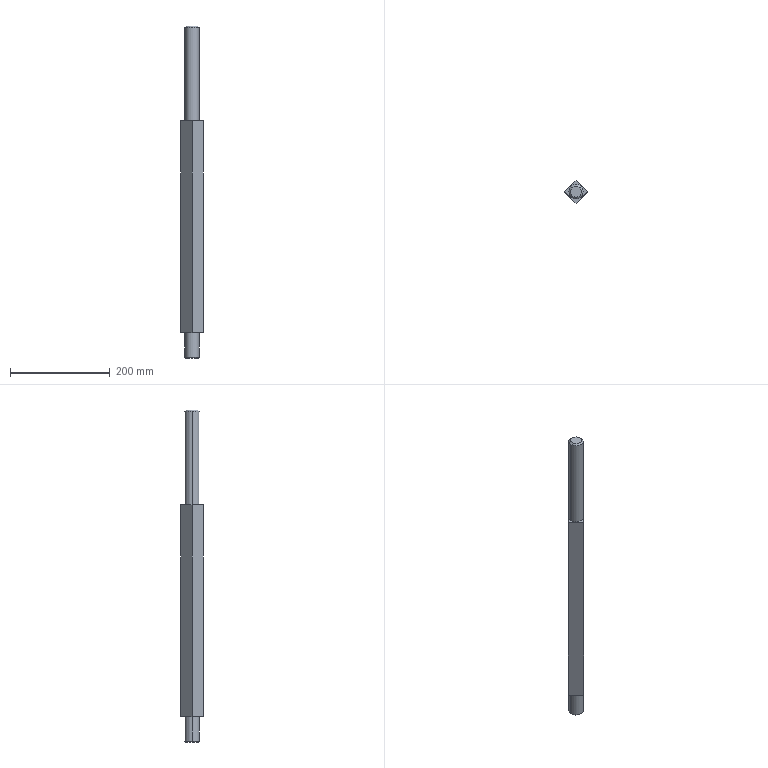Part | SolidWorks | features Chamfer 2, Extrusion 1, RevCut 1 | 1 solid | 16 faces | box 45.255 x 45.255 x 664.7 mm | volume 588102 mm3 | plane 8 | cone 4 | cylinder 4 | commonest cylinder face diameters 28.575 x4
STEP:
#1=CARTESIAN_POINT('',(11.287,0.,664.7));
#2=VERTEX_POINT('',#1);
#3=CARTESIAN_POINT('',(-11.287,0.,664.7));
#4=VERTEX_POINT('',#3);
#5=CARTESIAN_POINT('',(0.,0.,664.7));
#6=DIRECTION('',(0.,0.,1.));
#7=DIRECTION('',(1.,0.,0.));
#8=AXIS2_PLACEMENT_3D('',#5,#6,#7);
#9=CIRCLE('',#8,11.287);
#10=EDGE_CURVE('',#2,#4,#9,.T.);
#11=ORIENTED_EDGE('',*,*,#10,.F.);
#12=CARTESIAN_POINT('',(14.288,0.,661.7));
#13=VERTEX_POINT('',#12);
#14=CARTESIAN_POINT('',(14.288,0.,661.7));
#15=DIRECTION('',(0.7071,0.,-0.7071));
#16=VECTOR('',#15,1000.);
#17=LINE('',#14,#16);
#18=EDGE_CURVE('',#2,#13,#17,.T.);
#19=ORIENTED_EDGE('',*,*,#18,.T.);
#20=CARTESIAN_POINT('',(-14.288,0.,661.7));
#21=VERTEX_POINT('',#20);
#22=CARTESIAN_POINT('',(0.,0.,661.7));
#23=DIRECTION('',(0.,0.,-1.));
#24=DIRECTION('',(1.,0.,0.));
#25=AXIS2_PLACEMENT_3D('',#22,#23,#24);
#26=CIRCLE('',#25,14.288);
#27=EDGE_CURVE('',#21,#13,#26,.T.);
#28=ORIENTED_EDGE('',*,*,#27,.F.);
#29=CARTESIAN_POINT('',(-14.288,0.,661.7));
#30=DIRECTION('',(-0.7071,0.,-0.7071));
#31=VECTOR('',#30,1000.);
#32=LINE('',#29,#31);
#33=EDGE_CURVE('',#4,#21,#32,.T.);
#34=ORIENTED_EDGE('',*,*,#33,.F.);
#35=EDGE_LOOP('',(#11,#19,#28,#34));
#36=FACE_OUTER_BOUND('',#35,.T.);
#37=CARTESIAN_POINT('',(0.,0.,661.7));
#38=DIRECTION('',(0.,0.,-1.));
#39=DIRECTION('',(-1.,0.,0.));
#40=AXIS2_PLACEMENT_3D('',#37,#38,#39);
#41=CONICAL_SURFACE('',#40,14.288,0.7854);
#42=ADVANCED_FACE('',(#36),#41,.T.);
#43=CARTESIAN_POINT('',(-12.787,0.,0.));
#44=VERTEX_POINT('',#43);
#45=CARTESIAN_POINT('',(12.787,0.,0.));
#46=VERTEX_POINT('',#45);
#47=CARTESIAN_POINT('',(0.,0.,0.));
#48=DIRECTION('',(0.,0.,-1.));
#49=DIRECTION('',(1.,0.,0.));
#50=AXIS2_PLACEMENT_3D('',#47,#48,#49);
#51=CIRCLE('',#50,12.787);
#52=EDGE_CURVE('',#44,#46,#51,.T.);
#53=ORIENTED_EDGE('',*,*,#52,.F.);
#54=CARTESIAN_POINT('',(-14.288,0.,1.5));
#55=VERTEX_POINT('',#54);
#56=CARTESIAN_POINT('',(-12.787,0.,0.));
#57=DIRECTION('',(-0.7071,0.,0.7071));
#58=VECTOR('',#57,1000.);
#59=LINE('',#56,#58);
#60=EDGE_CURVE('',#44,#55,#59,.T.);
#61=ORIENTED_EDGE('',*,*,#60,.T.);
#62=CARTESIAN_POINT('',(14.288,0.,1.5));
#63=VERTEX_POINT('',#62);
#64=CARTESIAN_POINT('',(0.,0.,1.5));
#65=DIRECTION('',(0.,0.,1.));
#66=DIRECTION('',(1.,0.,0.));
#67=AXIS2_PLACEMENT_3D('',#64,#65,#66);
#68=CIRCLE('',#67,14.288);
#69=EDGE_CURVE('',#63,#55,#68,.T.);
#70=ORIENTED_EDGE('',*,*,#69,.F.);
#71=CARTESIAN_POINT('',(12.787,0.,0.));
#72=DIRECTION('',(0.7071,0.,0.7071));
#73=VECTOR('',#72,1000.);
#74=LINE('',#71,#73);
#75=EDGE_CURVE('',#46,#63,#74,.T.);
#76=ORIENTED_EDGE('',*,*,#75,.F.);
#77=EDGE_LOOP('',(#53,#61,#70,#76));
#78=FACE_OUTER_BOUND('',#77,.T.);
#79=CARTESIAN_POINT('',(0.,0.,0.));
#80=DIRECTION('',(0.,0.,1.));
#81=DIRECTION('',(1.,0.,0.));
#82=AXIS2_PLACEMENT_3D('',#79,#80,#81);
#83=CONICAL_SURFACE('',#82,12.787,0.7854);
#84=ADVANCED_FACE('',(#78),#83,.T.);
#85=ORIENTED_EDGE('',*,*,#27,.T.);
#86=CARTESIAN_POINT('',(14.288,0.,474.9));
#87=VERTEX_POINT('',#86);
#88=CARTESIAN_POINT('',(14.288,0.,0.));
#89=DIRECTION('',(0.,0.,-1.));
#90=VECTOR('',#89,1000.);
#91=LINE('',#88,#90);
#92=EDGE_CURVE('',#13,#87,#91,.T.);
#93=ORIENTED_EDGE('',*,*,#92,.T.);
#94=CARTESIAN_POINT('',(-14.288,0.,474.9));
#95=VERTEX_POINT('',#94);
#96=CARTESIAN_POINT('',(0.,0.,474.9));
#97=DIRECTION('',(0.,0.,-1.));
#98=DIRECTION('',(-1.,0.,0.));
#99=AXIS2_PLACEMENT_3D('',#96,#97,#98);
#100=CIRCLE('',#99,14.288);
#101=EDGE_CURVE('',#95,#87,#100,.T.);
#102=ORIENTED_EDGE('',*,*,#101,.F.);
#103=CARTESIAN_POINT('',(-14.288,0.,0.));
#104=DIRECTION('',(0.,0.,-1.));
#105=VECTOR('',#104,1000.);
#106=LINE('',#103,#105);
#107=EDGE_CURVE('',#21,#95,#106,.T.);
#108=ORIENTED_EDGE('',*,*,#107,.F.);
#109=EDGE_LOOP('',(#85,#93,#102,#108));
#110=FACE_OUTER_BOUND('',#109,.T.);
#111=CARTESIAN_POINT('',(0.,0.,0.));
#112=DIRECTION('',(0.,0.,-1.));
#113=DIRECTION('',(-1.,0.,0.));
#114=AXIS2_PLACEMENT_3D('',#111,#112,#113);
#115=CYLINDRICAL_SURFACE('',#114,14.288);
#116=ADVANCED_FACE('',(#110),#115,.T.);
#117=CARTESIAN_POINT('',(-14.288,0.,50.8));
#118=VERTEX_POINT('',#117);
#119=CARTESIAN_POINT('',(14.288,0.,50.8));
#120=VERTEX_POINT('',#119);
#121=CARTESIAN_POINT('',(0.,0.,50.8));
#122=DIRECTION('',(0.,0.,-1.));
#123=DIRECTION('',(-1.,0.,0.));
#124=AXIS2_PLACEMENT_3D('',#121,#122,#123);
#125=CIRCLE('',#124,14.288);
#126=EDGE_CURVE('',#118,#120,#125,.T.);
#127=ORIENTED_EDGE('',*,*,#126,.T.);
#128=CARTESIAN_POINT('',(14.288,0.,0.));
#129=DIRECTION('',(0.,0.,-1.));
#130=VECTOR('',#129,1000.);
#131=LINE('',#128,#130);
#132=EDGE_CURVE('',#120,#63,#131,.T.);
#133=ORIENTED_EDGE('',*,*,#132,.T.);
#134=ORIENTED_EDGE('',*,*,#69,.T.);
#135=CARTESIAN_POINT('',(-14.288,0.,0.));
#136=DIRECTION('',(0.,0.,-1.));
#137=VECTOR('',#136,1000.);
#138=LINE('',#135,#137);
#139=EDGE_CURVE('',#118,#55,#138,.T.);
#140=ORIENTED_EDGE('',*,*,#139,.F.);
#141=EDGE_LOOP('',(#127,#133,#134,#140));
#142=FACE_OUTER_BOUND('',#141,.T.);
#143=CARTESIAN_POINT('',(0.,0.,0.));
#144=DIRECTION('',(0.,0.,-1.));
#145=DIRECTION('',(-1.,0.,0.));
#146=AXIS2_PLACEMENT_3D('',#143,#144,#145);
#147=CYLINDRICAL_SURFACE('',#146,14.288);
#148=ADVANCED_FACE('',(#142),#147,.T.);
#149=CARTESIAN_POINT('',(-22.627,0.,474.9));
#150=VERTEX_POINT('',#149);
#151=CARTESIAN_POINT('',(0.,-22.627,474.9));
#152=VERTEX_POINT('',#151);
#153=CARTESIAN_POINT('',(-22.627,0.,474.9));
#154=DIRECTION('',(0.7071,-0.7071,0.));
#155=VECTOR('',#154,1000.);
#156=LINE('',#153,#155);
#157=EDGE_CURVE('',#150,#152,#156,.T.);
#158=ORIENTED_EDGE('',*,*,#157,.F.);
#159=CARTESIAN_POINT('',(-22.627,0.,50.8));
#160=VERTEX_POINT('',#159);
#161=CARTESIAN_POINT('',(-22.627,0.,664.7));
#162=DIRECTION('',(0.,0.,-1.));
#163=VECTOR('',#162,1000.);
#164=LINE('',#161,#163);
#165=EDGE_CURVE('',#150,#160,#164,.T.);
#166=ORIENTED_EDGE('',*,*,#165,.T.);
#167=CARTESIAN_POINT('',(0.,-22.627,50.8));
#168=VERTEX_POINT('',#167);
#169=CARTESIAN_POINT('',(-22.627,0.,50.8));
#170=DIRECTION('',(-0.7071,0.7071,0.));
#171=VECTOR('',#170,1000.);
#172=LINE('',#169,#171);
#173=EDGE_CURVE('',#168,#160,#172,.T.);
#174=ORIENTED_EDGE('',*,*,#173,.F.);
#175=CARTESIAN_POINT('',(0.,-22.627,664.7));
#176=DIRECTION('',(0.,0.,-1.));
#177=VECTOR('',#176,1000.);
#178=LINE('',#175,#177);
#179=EDGE_CURVE('',#152,#168,#178,.T.);
#180=ORIENTED_EDGE('',*,*,#179,.F.);
#181=EDGE_LOOP('',(#158,#166,#174,#180));
#182=FACE_OUTER_BOUND('',#181,.T.);
#183=CARTESIAN_POINT('',(-22.627,0.,664.7));
#184=DIRECTION('',(0.7071,0.7071,0.));
#185=DIRECTION('',(-0.7071,0.7071,0.));
#186=AXIS2_PLACEMENT_3D('',#183,#184,#185);
#187=PLANE('',#186);
#188=ADVANCED_FACE('',(#182),#187,.F.);
#189=CARTESIAN_POINT('',(22.627,0.,474.9));
#190=VERTEX_POINT('',#189);
#191=CARTESIAN_POINT('',(0.,-22.627,474.9));
#192=DIRECTION('',(0.7071,0.7071,0.));
#193=VECTOR('',#192,1000.);
#194=LINE('',#191,#193);
#195=EDGE_CURVE('',#152,#190,#194,.T.);
#196=ORIENTED_EDGE('',*,*,#195,.F.);
#197=ORIENTED_EDGE('',*,*,#179,.T.);
#198=CARTESIAN_POINT('',(22.627,0.,50.8));
#199=VERTEX_POINT('',#198);
#200=CARTESIAN_POINT('',(0.,-22.627,50.8));
#201=DIRECTION('',(-0.7071,-0.7071,0.));
#202=VECTOR('',#201,1000.);
#203=LINE('',#200,#202);
#204=EDGE_CURVE('',#199,#168,#203,.T.);
#205=ORIENTED_EDGE('',*,*,#204,.F.);
#206=CARTESIAN_POINT('',(22.627,0.,664.7));
#207=DIRECTION('',(0.,0.,-1.));
#208=VECTOR('',#207,1000.);
#209=LINE('',#206,#208);
#210=EDGE_CURVE('',#190,#199,#209,.T.);
#211=ORIENTED_EDGE('',*,*,#210,.F.);
#212=EDGE_LOOP('',(#196,#197,#205,#211));
#213=FACE_OUTER_BOUND('',#212,.T.);
#214=CARTESIAN_POINT('',(0.,-22.627,664.7));
#215=DIRECTION('',(-0.7071,0.7071,0.));
#216=DIRECTION('',(-0.7071,-0.7071,0.));
#217=AXIS2_PLACEMENT_3D('',#214,#215,#216);
#218=PLANE('',#217);
#219=ADVANCED_FACE('',(#213),#218,.F.);
#220=CARTESIAN_POINT('',(0.,22.627,474.9));
#221=VERTEX_POINT('',#220);
#222=CARTESIAN_POINT('',(0.,22.627,474.9));
#223=DIRECTION('',(-0.7071,0.7071,0.));
#224=VECTOR('',#223,1000.);
#225=LINE('',#222,#224);
#226=EDGE_CURVE('',#190,#221,#225,.T.);
#227=ORIENTED_EDGE('',*,*,#226,.F.);
#228=ORIENTED_EDGE('',*,*,#210,.T.);
#229=CARTESIAN_POINT('',(0.,22.627,50.8));
#230=VERTEX_POINT('',#229);
#231=CARTESIAN_POINT('',(0.,22.627,50.8));
#232=DIRECTION('',(0.7071,-0.7071,0.));
#233=VECTOR('',#232,1000.);
#234=LINE('',#231,#233);
#235=EDGE_CURVE('',#230,#199,#234,.T.);
#236=ORIENTED_EDGE('',*,*,#235,.F.);
#237=CARTESIAN_POINT('',(0.,22.627,664.7));
#238=DIRECTION('',(0.,0.,-1.));
#239=VECTOR('',#238,1000.);
#240=LINE('',#237,#239);
#241=EDGE_CURVE('',#221,#230,#240,.T.);
#242=ORIENTED_EDGE('',*,*,#241,.F.);
#243=EDGE_LOOP('',(#227,#228,#236,#242));
#244=FACE_OUTER_BOUND('',#243,.T.);
#245=CARTESIAN_POINT('',(0.,22.627,664.7));
#246=DIRECTION('',(-0.7071,-0.7071,0.));
#247=DIRECTION('',(0.7071,-0.7071,0.));
#248=AXIS2_PLACEMENT_3D('',#245,#246,#247);
#249=PLANE('',#248);
#250=ADVANCED_FACE('',(#244),#249,.F.);
#251=CARTESIAN_POINT('',(-22.627,0.,474.9));
#252=DIRECTION('',(-0.7071,-0.7071,0.));
#253=VECTOR('',#252,1000.);
#254=LINE('',#251,#253);
#255=EDGE_CURVE('',#221,#150,#254,.T.);
#256=ORIENTED_EDGE('',*,*,#255,.F.);
#257=ORIENTED_EDGE('',*,*,#241,.T.);
#258=CARTESIAN_POINT('',(-22.627,0.,50.8));
#259=DIRECTION('',(0.7071,0.7071,0.));
#260=VECTOR('',#259,1000.);
#261=LINE('',#258,#260);
#262=EDGE_CURVE('',#160,#230,#261,.T.);
#263=ORIENTED_EDGE('',*,*,#262,.F.);
#264=ORIENTED_EDGE('',*,*,#165,.F.);
#265=EDGE_LOOP('',(#256,#257,#263,#264));
#266=FACE_OUTER_BOUND('',#265,.T.);
#267=CARTESIAN_POINT('',(-22.627,0.,664.7));
#268=DIRECTION('',(0.7071,-0.7071,0.));
#269=DIRECTION('',(0.7071,0.7071,0.));
#270=AXIS2_PLACEMENT_3D('',#267,#268,#269);
#271=PLANE('',#270);
#272=ADVANCED_FACE('',(#266),#271,.F.);
#273=ORIENTED_EDGE('',*,*,#126,.F.);
#274=CARTESIAN_POINT('',(0.,0.,50.8));
#275=DIRECTION('',(0.,0.,-1.));
#276=DIRECTION('',(-1.,0.,0.));
#277=AXIS2_PLACEMENT_3D('',#274,#275,#276);
#278=CIRCLE('',#277,14.288);
#279=EDGE_CURVE('',#120,#118,#278,.T.);
#280=ORIENTED_EDGE('',*,*,#279,.F.);
#281=EDGE_LOOP('',(#273,#280));
#282=FACE_BOUND('',#281,.T.);
#283=ORIENTED_EDGE('',*,*,#173,.T.);
#284=ORIENTED_EDGE('',*,*,#262,.T.);
#285=ORIENTED_EDGE('',*,*,#235,.T.);
#286=ORIENTED_EDGE('',*,*,#204,.T.);
#287=EDGE_LOOP('',(#283,#284,#285,#286));
#288=FACE_OUTER_BOUND('',#287,.T.);
#289=CARTESIAN_POINT('',(14.288,0.,50.8));
#290=DIRECTION('',(0.,0.,-1.));
#291=DIRECTION('',(-1.,0.,0.));
#292=AXIS2_PLACEMENT_3D('',#289,#290,#291);
#293=PLANE('',#292);
#294=ADVANCED_FACE('',(#282,#288),#293,.T.);
#295=ORIENTED_EDGE('',*,*,#132,.F.);
#296=ORIENTED_EDGE('',*,*,#279,.T.);
#297=ORIENTED_EDGE('',*,*,#139,.T.);
#298=CARTESIAN_POINT('',(0.,0.,1.5));
#299=DIRECTION('',(0.,0.,1.));
#300=DIRECTION('',(1.,0.,0.));
#301=AXIS2_PLACEMENT_3D('',#298,#299,#300);
#302=CIRCLE('',#301,14.288);
#303=EDGE_CURVE('',#55,#63,#302,.T.);
#304=ORIENTED_EDGE('',*,*,#303,.T.);
#305=EDGE_LOOP('',(#295,#296,#297,#304));
#306=FACE_OUTER_BOUND('',#305,.T.);
#307=CARTESIAN_POINT('',(0.,0.,0.));
#308=DIRECTION('',(0.,0.,-1.));
#309=DIRECTION('',(-1.,0.,0.));
#310=AXIS2_PLACEMENT_3D('',#307,#308,#309);
#311=CYLINDRICAL_SURFACE('',#310,14.288);
#312=ADVANCED_FACE('',(#306),#311,.T.);
#313=CARTESIAN_POINT('',(0.,0.,0.));
#314=DIRECTION('',(0.,0.,-1.));
#315=DIRECTION('',(1.,0.,0.));
#316=AXIS2_PLACEMENT_3D('',#313,#314,#315);
#317=CIRCLE('',#316,12.787);
#318=EDGE_CURVE('',#46,#44,#317,.T.);
#319=ORIENTED_EDGE('',*,*,#318,.T.);
#320=ORIENTED_EDGE('',*,*,#52,.T.);
#321=EDGE_LOOP('',(#319,#320));
#322=FACE_OUTER_BOUND('',#321,.T.);
#323=CARTESIAN_POINT('',(0.,-22.627,0.));
#324=DIRECTION('',(0.,0.,1.));
#325=DIRECTION('',(1.,0.,0.));
#326=AXIS2_PLACEMENT_3D('',#323,#324,#325);
#327=PLANE('',#326);
#328=ADVANCED_FACE('',(#322),#327,.F.);
#329=ORIENTED_EDGE('',*,*,#101,.T.);
#330=CARTESIAN_POINT('',(0.,0.,474.9));
#331=DIRECTION('',(0.,0.,-1.));
#332=DIRECTION('',(-1.,0.,0.));
#333=AXIS2_PLACEMENT_3D('',#330,#331,#332);
#334=CIRCLE('',#333,14.288);
#335=EDGE_CURVE('',#87,#95,#334,.T.);
#336=ORIENTED_EDGE('',*,*,#335,.T.);
#337=EDGE_LOOP('',(#329,#336));
#338=FACE_BOUND('',#337,.T.);
#339=ORIENTED_EDGE('',*,*,#157,.T.);
#340=ORIENTED_EDGE('',*,*,#195,.T.);
#341=ORIENTED_EDGE('',*,*,#226,.T.);
#342=ORIENTED_EDGE('',*,*,#255,.T.);
#343=EDGE_LOOP('',(#339,#340,#341,#342));
#344=FACE_OUTER_BOUND('',#343,.T.);
#345=CARTESIAN_POINT('',(14.288,0.,474.9));
#346=DIRECTION('',(0.,0.,1.));
#347=DIRECTION('',(1.,0.,0.));
#348=AXIS2_PLACEMENT_3D('',#345,#346,#347);
#349=PLANE('',#348);
#350=ADVANCED_FACE('',(#338,#344),#349,.T.);
#351=ORIENTED_EDGE('',*,*,#92,.F.);
#352=CARTESIAN_POINT('',(0.,0.,661.7));
#353=DIRECTION('',(0.,0.,-1.));
#354=DIRECTION('',(1.,0.,0.));
#355=AXIS2_PLACEMENT_3D('',#352,#353,#354);
#356=CIRCLE('',#355,14.288);
#357=EDGE_CURVE('',#13,#21,#356,.T.);
#358=ORIENTED_EDGE('',*,*,#357,.T.);
#359=ORIENTED_EDGE('',*,*,#107,.T.);
#360=ORIENTED_EDGE('',*,*,#335,.F.);
#361=EDGE_LOOP('',(#351,#358,#359,#360));
#362=FACE_OUTER_BOUND('',#361,.T.);
#363=CARTESIAN_POINT('',(0.,0.,0.));
#364=DIRECTION('',(0.,0.,-1.));
#365=DIRECTION('',(-1.,0.,0.));
#366=AXIS2_PLACEMENT_3D('',#363,#364,#365);
#367=CYLINDRICAL_SURFACE('',#366,14.288);
#368=ADVANCED_FACE('',(#362),#367,.T.);
#369=CARTESIAN_POINT('',(0.,0.,664.7));
#370=DIRECTION('',(0.,0.,1.));
#371=DIRECTION('',(1.,0.,0.));
#372=AXIS2_PLACEMENT_3D('',#369,#370,#371);
#373=CIRCLE('',#372,11.287);
#374=EDGE_CURVE('',#4,#2,#373,.T.);
#375=ORIENTED_EDGE('',*,*,#374,.T.);
#376=ORIENTED_EDGE('',*,*,#10,.T.);
#377=EDGE_LOOP('',(#375,#376));
#378=FACE_OUTER_BOUND('',#377,.T.);
#379=CARTESIAN_POINT('',(0.,-22.627,664.7));
#380=DIRECTION('',(0.,0.,1.));
#381=DIRECTION('',(1.,0.,0.));
#382=AXIS2_PLACEMENT_3D('',#379,#380,#381);
#383=PLANE('',#382);
#384=ADVANCED_FACE('',(#378),#383,.T.);
#385=ORIENTED_EDGE('',*,*,#60,.F.);
#386=ORIENTED_EDGE('',*,*,#318,.F.);
#387=ORIENTED_EDGE('',*,*,#75,.T.);
#388=ORIENTED_EDGE('',*,*,#303,.F.);
#389=EDGE_LOOP('',(#385,#386,#387,#388));
#390=FACE_OUTER_BOUND('',#389,.T.);
#391=CARTESIAN_POINT('',(0.,0.,0.));
#392=DIRECTION('',(0.,0.,1.));
#393=DIRECTION('',(1.,0.,0.));
#394=AXIS2_PLACEMENT_3D('',#391,#392,#393);
#395=CONICAL_SURFACE('',#394,12.787,0.7854);
#396=ADVANCED_FACE('',(#390),#395,.T.);
#397=ORIENTED_EDGE('',*,*,#18,.F.);
#398=ORIENTED_EDGE('',*,*,#374,.F.);
#399=ORIENTED_EDGE('',*,*,#33,.T.);
#400=ORIENTED_EDGE('',*,*,#357,.F.);
#401=EDGE_LOOP('',(#397,#398,#399,#400));
#402=FACE_OUTER_BOUND('',#401,.T.);
#403=CARTESIAN_POINT('',(0.,0.,661.7));
#404=DIRECTION('',(0.,0.,-1.));
#405=DIRECTION('',(-1.,0.,0.));
#406=AXIS2_PLACEMENT_3D('',#403,#404,#405);
#407=CONICAL_SURFACE('',#406,14.288,0.7854);
#408=ADVANCED_FACE('',(#402),#407,.T.);
#409=CLOSED_SHELL('',(#42,#84,#116,#148,#188,#219,#250,#272,#294,#312,#328,#350,#368,#384,#396,#408));
#410=MANIFOLD_SOLID_BREP('',#409);
#411=CARTESIAN_POINT('',(0.,0.,0.));
#412=DIRECTION('',(0.,0.,1.));
#413=DIRECTION('',(1.,0.,0.));
#414=AXIS2_PLACEMENT_3D('',#411,#412,#413);
#415=(LENGTH_UNIT()NAMED_UNIT(*)SI_UNIT(.MILLI.,.METRE.));
#416=UNCERTAINTY_MEASURE_WITH_UNIT(LENGTH_MEASURE(0.00001),#415,'','');
#417=(NAMED_UNIT(*)PLANE_ANGLE_UNIT()SI_UNIT($,.RADIAN.));
#418=(NAMED_UNIT(*)SI_UNIT($,.STERADIAN.)SOLID_ANGLE_UNIT());
#419=(GEOMETRIC_REPRESENTATION_CONTEXT(3)GLOBAL_UNCERTAINTY_ASSIGNED_CONTEXT((#416))GLOBAL_UNIT_ASSIGNED_CONTEXT((#415,#417,#418))REPRESENTATION_CONTEXT('',''));
#420=ADVANCED_BREP_SHAPE_REPRESENTATION('',(#410,#414),#419);